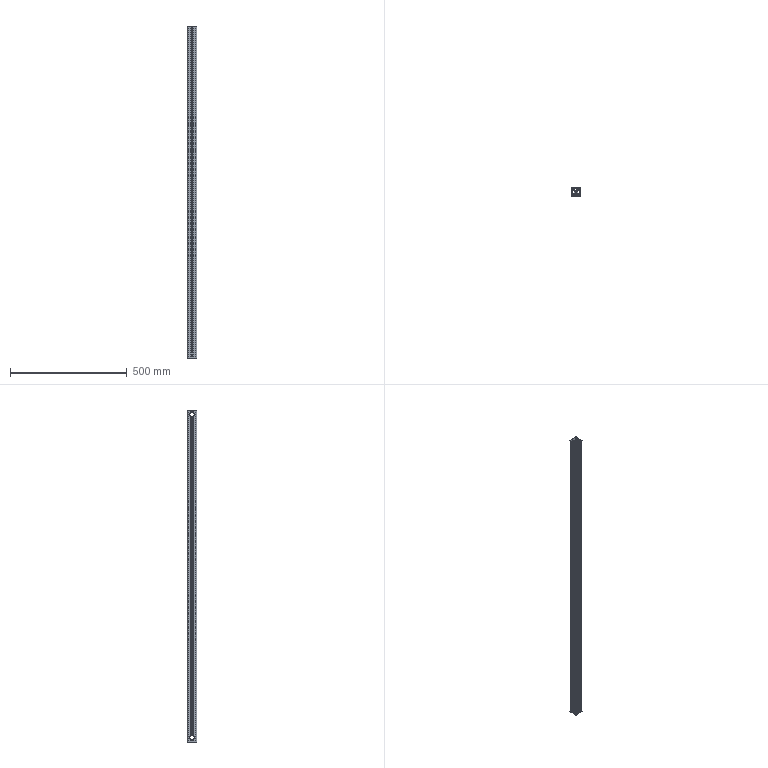Part | SolidWorks | features BaseBody 1, HoleWzd 1, MoveFace 1 | 1 solid | 242 faces | box 40 x 40 x 1420 mm | volume 832360 mm3 | plane 187 | cylinder 55 | commonest cylinder face diameters 6.8 x15 2 x14 19 x12 1 x6 5 x4 9 x4